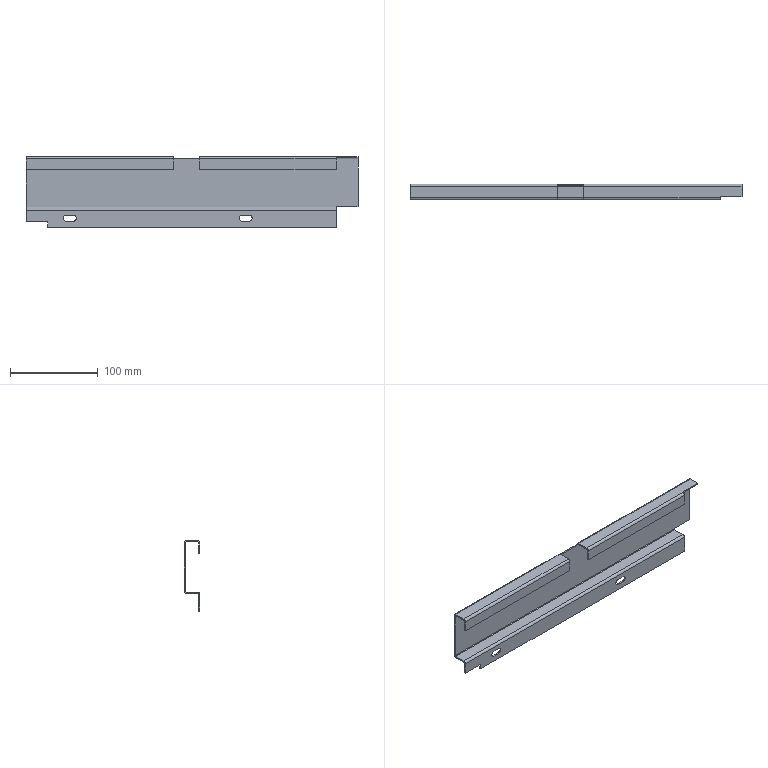Part | STEP file | 1 solid | 62 faces | box 378 x 18 x 80.5 mm | volume 66341 mm3 | plane 46 | cylinder 16 | commonest cylinder face diameters 2 x6 5 x6 7 x4